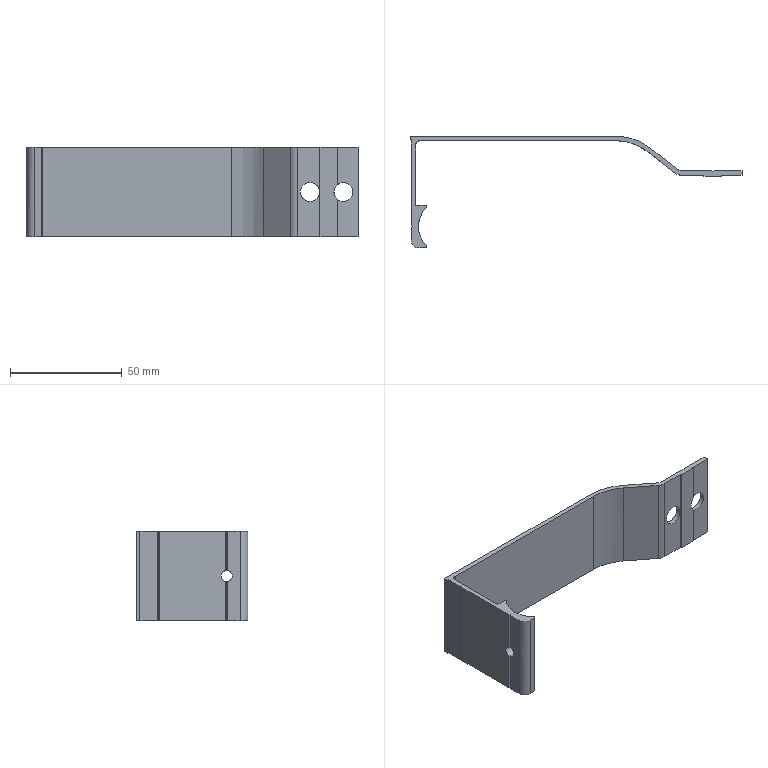Part | STEP file | 31E-01001QY15 | 1 solid | 49 faces | box 148.5 x 50 x 40 mm | volume 17812 mm3 | plane 31 | cylinder 18 | commonest cylinder face diameters 1 x4 8.5 x4 5 x2 25.4 x2 4 x1 6 x1